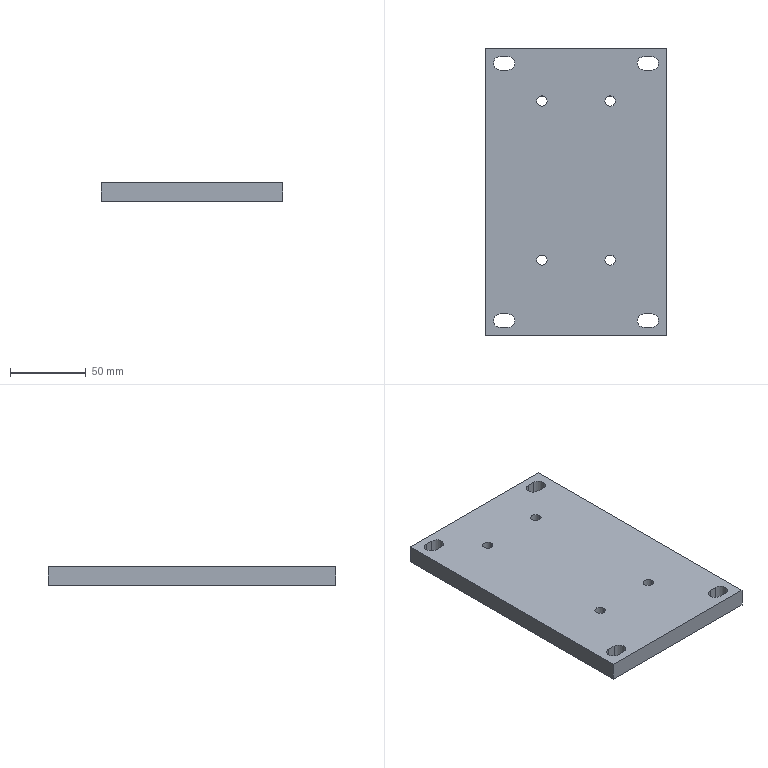Part | STEP file | X77-08202 | 1 solid | 44 faces | box 120 x 190 x 12 mm | volume 260641 mm3 | cylinder 24 | plane 20 | commonest cylinder face diameters 9 x12 6.8 x8 8 x4
STEP:
#1=CARTESIAN_POINT('',(25.9,-643.608,12.));
#2=VERTEX_POINT('',#1);
#3=CARTESIAN_POINT('',(19.1,-643.608,12.));
#4=VERTEX_POINT('',#3);
#5=CARTESIAN_POINT('',(22.5,-643.608,12.));
#6=DIRECTION('',(0.,0.,-1.));
#7=DIRECTION('',(-1.,0.,0.));
#8=AXIS2_PLACEMENT_3D('',#5,#6,#7);
#9=CIRCLE('',#8,3.4);
#10=EDGE_CURVE('',#2,#4,#9,.T.);
#11=ORIENTED_EDGE('',*,*,#10,.F.);
#12=CARTESIAN_POINT('',(25.9,-643.608,2.5));
#13=VERTEX_POINT('',#12);
#14=CARTESIAN_POINT('',(25.9,-643.608,2.5));
#15=DIRECTION('',(0.,0.,-1.));
#16=VECTOR('',#15,1000.);
#17=LINE('',#14,#16);
#18=EDGE_CURVE('',#2,#13,#17,.T.);
#19=ORIENTED_EDGE('',*,*,#18,.T.);
#20=CARTESIAN_POINT('',(19.1,-643.608,2.5));
#21=VERTEX_POINT('',#20);
#22=CARTESIAN_POINT('',(22.5,-643.608,2.5));
#23=DIRECTION('',(0.,0.,-1.));
#24=DIRECTION('',(-1.,0.,0.));
#25=AXIS2_PLACEMENT_3D('',#22,#23,#24);
#26=CIRCLE('',#25,3.4);
#27=EDGE_CURVE('',#13,#21,#26,.T.);
#28=ORIENTED_EDGE('',*,*,#27,.T.);
#29=CARTESIAN_POINT('',(19.1,-643.608,2.5));
#30=DIRECTION('',(0.,0.,-1.));
#31=VECTOR('',#30,1000.);
#32=LINE('',#29,#31);
#33=EDGE_CURVE('',#4,#21,#32,.T.);
#34=ORIENTED_EDGE('',*,*,#33,.F.);
#35=EDGE_LOOP('',(#11,#19,#28,#34));
#36=FACE_OUTER_BOUND('',#35,.T.);
#37=CARTESIAN_POINT('',(22.5,-643.608,2.5));
#38=DIRECTION('',(0.,0.,-1.));
#39=DIRECTION('',(-1.,0.,0.));
#40=AXIS2_PLACEMENT_3D('',#37,#38,#39);
#41=CYLINDRICAL_SURFACE('',#40,3.4);
#42=ADVANCED_FACE('',(#36),#41,.F.);
#43=CARTESIAN_POINT('',(-19.1,-643.601,12.));
#44=VERTEX_POINT('',#43);
#45=CARTESIAN_POINT('',(-25.9,-643.601,12.));
#46=VERTEX_POINT('',#45);
#47=CARTESIAN_POINT('',(-22.5,-643.601,12.));
#48=DIRECTION('',(0.,0.,-1.));
#49=DIRECTION('',(-1.,0.,0.));
#50=AXIS2_PLACEMENT_3D('',#47,#48,#49);
#51=CIRCLE('',#50,3.4);
#52=EDGE_CURVE('',#44,#46,#51,.T.);
#53=ORIENTED_EDGE('',*,*,#52,.F.);
#54=CARTESIAN_POINT('',(-19.1,-643.601,2.5));
#55=VERTEX_POINT('',#54);
#56=CARTESIAN_POINT('',(-19.1,-643.601,2.5));
#57=DIRECTION('',(0.,0.,-1.));
#58=VECTOR('',#57,1000.);
#59=LINE('',#56,#58);
#60=EDGE_CURVE('',#44,#55,#59,.T.);
#61=ORIENTED_EDGE('',*,*,#60,.T.);
#62=CARTESIAN_POINT('',(-25.9,-643.601,2.5));
#63=VERTEX_POINT('',#62);
#64=CARTESIAN_POINT('',(-22.5,-643.601,2.5));
#65=DIRECTION('',(0.,0.,-1.));
#66=DIRECTION('',(-1.,0.,0.));
#67=AXIS2_PLACEMENT_3D('',#64,#65,#66);
#68=CIRCLE('',#67,3.4);
#69=EDGE_CURVE('',#55,#63,#68,.T.);
#70=ORIENTED_EDGE('',*,*,#69,.T.);
#71=CARTESIAN_POINT('',(-25.9,-643.601,2.5));
#72=DIRECTION('',(0.,0.,-1.));
#73=VECTOR('',#72,1000.);
#74=LINE('',#71,#73);
#75=EDGE_CURVE('',#46,#63,#74,.T.);
#76=ORIENTED_EDGE('',*,*,#75,.F.);
#77=EDGE_LOOP('',(#53,#61,#70,#76));
#78=FACE_OUTER_BOUND('',#77,.T.);
#79=CARTESIAN_POINT('',(-22.5,-643.601,2.5));
#80=DIRECTION('',(0.,0.,-1.));
#81=DIRECTION('',(-1.,0.,0.));
#82=AXIS2_PLACEMENT_3D('',#79,#80,#81);
#83=CYLINDRICAL_SURFACE('',#82,3.4);
#84=ADVANCED_FACE('',(#78),#83,.F.);
#85=CARTESIAN_POINT('',(-19.1,-538.608,12.));
#86=VERTEX_POINT('',#85);
#87=CARTESIAN_POINT('',(-25.9,-538.608,12.));
#88=VERTEX_POINT('',#87);
#89=CARTESIAN_POINT('',(-22.5,-538.608,12.));
#90=DIRECTION('',(0.,0.,-1.));
#91=DIRECTION('',(-1.,0.,0.));
#92=AXIS2_PLACEMENT_3D('',#89,#90,#91);
#93=CIRCLE('',#92,3.4);
#94=EDGE_CURVE('',#86,#88,#93,.T.);
#95=ORIENTED_EDGE('',*,*,#94,.F.);
#96=CARTESIAN_POINT('',(-19.1,-538.608,2.5));
#97=VERTEX_POINT('',#96);
#98=CARTESIAN_POINT('',(-19.1,-538.608,2.5));
#99=DIRECTION('',(0.,0.,-1.));
#100=VECTOR('',#99,1000.);
#101=LINE('',#98,#100);
#102=EDGE_CURVE('',#86,#97,#101,.T.);
#103=ORIENTED_EDGE('',*,*,#102,.T.);
#104=CARTESIAN_POINT('',(-25.9,-538.608,2.5));
#105=VERTEX_POINT('',#104);
#106=CARTESIAN_POINT('',(-22.5,-538.608,2.5));
#107=DIRECTION('',(0.,0.,-1.));
#108=DIRECTION('',(-1.,0.,0.));
#109=AXIS2_PLACEMENT_3D('',#106,#107,#108);
#110=CIRCLE('',#109,3.4);
#111=EDGE_CURVE('',#97,#105,#110,.T.);
#112=ORIENTED_EDGE('',*,*,#111,.T.);
#113=CARTESIAN_POINT('',(-25.9,-538.608,2.5));
#114=DIRECTION('',(0.,0.,-1.));
#115=VECTOR('',#114,1000.);
#116=LINE('',#113,#115);
#117=EDGE_CURVE('',#88,#105,#116,.T.);
#118=ORIENTED_EDGE('',*,*,#117,.F.);
#119=EDGE_LOOP('',(#95,#103,#112,#118));
#120=FACE_OUTER_BOUND('',#119,.T.);
#121=CARTESIAN_POINT('',(-22.5,-538.608,2.5));
#122=DIRECTION('',(0.,0.,-1.));
#123=DIRECTION('',(-1.,0.,0.));
#124=AXIS2_PLACEMENT_3D('',#121,#122,#123);
#125=CYLINDRICAL_SURFACE('',#124,3.4);
#126=ADVANCED_FACE('',(#120),#125,.F.);
#127=CARTESIAN_POINT('',(25.9,-538.608,12.));
#128=VERTEX_POINT('',#127);
#129=CARTESIAN_POINT('',(19.1,-538.608,12.));
#130=VERTEX_POINT('',#129);
#131=CARTESIAN_POINT('',(22.5,-538.608,12.));
#132=DIRECTION('',(0.,0.,-1.));
#133=DIRECTION('',(-1.,0.,0.));
#134=AXIS2_PLACEMENT_3D('',#131,#132,#133);
#135=CIRCLE('',#134,3.4);
#136=EDGE_CURVE('',#128,#130,#135,.T.);
#137=ORIENTED_EDGE('',*,*,#136,.F.);
#138=CARTESIAN_POINT('',(25.9,-538.608,2.5));
#139=VERTEX_POINT('',#138);
#140=CARTESIAN_POINT('',(25.9,-538.608,2.5));
#141=DIRECTION('',(0.,0.,-1.));
#142=VECTOR('',#141,1000.);
#143=LINE('',#140,#142);
#144=EDGE_CURVE('',#128,#139,#143,.T.);
#145=ORIENTED_EDGE('',*,*,#144,.T.);
#146=CARTESIAN_POINT('',(19.1,-538.608,2.5));
#147=VERTEX_POINT('',#146);
#148=CARTESIAN_POINT('',(22.5,-538.608,2.5));
#149=DIRECTION('',(0.,0.,-1.));
#150=DIRECTION('',(-1.,0.,0.));
#151=AXIS2_PLACEMENT_3D('',#148,#149,#150);
#152=CIRCLE('',#151,3.4);
#153=EDGE_CURVE('',#139,#147,#152,.T.);
#154=ORIENTED_EDGE('',*,*,#153,.T.);
#155=CARTESIAN_POINT('',(19.1,-538.608,2.5));
#156=DIRECTION('',(0.,0.,-1.));
#157=VECTOR('',#156,1000.);
#158=LINE('',#155,#157);
#159=EDGE_CURVE('',#130,#147,#158,.T.);
#160=ORIENTED_EDGE('',*,*,#159,.F.);
#161=EDGE_LOOP('',(#137,#145,#154,#160));
#162=FACE_OUTER_BOUND('',#161,.T.);
#163=CARTESIAN_POINT('',(22.5,-538.608,2.5));
#164=DIRECTION('',(0.,0.,-1.));
#165=DIRECTION('',(-1.,0.,0.));
#166=AXIS2_PLACEMENT_3D('',#163,#164,#165);
#167=CYLINDRICAL_SURFACE('',#166,3.4);
#168=ADVANCED_FACE('',(#162),#167,.F.);
#169=CARTESIAN_POINT('',(-50.028,-679.108,12.));
#170=VERTEX_POINT('',#169);
#171=CARTESIAN_POINT('',(-54.528,-683.608,12.));
#172=VERTEX_POINT('',#171);
#173=CARTESIAN_POINT('',(-50.028,-683.608,12.));
#174=DIRECTION('',(0.,0.,1.));
#175=DIRECTION('',(-1.,0.,0.));
#176=AXIS2_PLACEMENT_3D('',#173,#174,#175);
#177=CIRCLE('',#176,4.5);
#178=EDGE_CURVE('',#170,#172,#177,.T.);
#179=ORIENTED_EDGE('',*,*,#178,.T.);
#180=CARTESIAN_POINT('',(-54.528,-683.608,0.));
#181=VERTEX_POINT('',#180);
#182=CARTESIAN_POINT('',(-54.528,-683.608,12.));
#183=DIRECTION('',(0.,0.,-1.));
#184=VECTOR('',#183,1000.);
#185=LINE('',#182,#184);
#186=EDGE_CURVE('',#172,#181,#185,.T.);
#187=ORIENTED_EDGE('',*,*,#186,.T.);
#188=CARTESIAN_POINT('',(-50.028,-679.108,0.));
#189=VERTEX_POINT('',#188);
#190=CARTESIAN_POINT('',(-50.028,-683.608,0.));
#191=DIRECTION('',(0.,0.,1.));
#192=DIRECTION('',(-1.,0.,0.));
#193=AXIS2_PLACEMENT_3D('',#190,#191,#192);
#194=CIRCLE('',#193,4.5);
#195=EDGE_CURVE('',#189,#181,#194,.T.);
#196=ORIENTED_EDGE('',*,*,#195,.F.);
#197=CARTESIAN_POINT('',(-50.028,-679.108,12.));
#198=DIRECTION('',(0.,0.,-1.));
#199=VECTOR('',#198,1000.);
#200=LINE('',#197,#199);
#201=EDGE_CURVE('',#170,#189,#200,.T.);
#202=ORIENTED_EDGE('',*,*,#201,.F.);
#203=EDGE_LOOP('',(#179,#187,#196,#202));
#204=FACE_OUTER_BOUND('',#203,.T.);
#205=CARTESIAN_POINT('',(-50.028,-683.608,12.));
#206=DIRECTION('',(0.,0.,-1.));
#207=DIRECTION('',(-1.,0.,0.));
#208=AXIS2_PLACEMENT_3D('',#205,#206,#207);
#209=CYLINDRICAL_SURFACE('',#208,4.5);
#210=ADVANCED_FACE('',(#204),#209,.F.);
#211=CARTESIAN_POINT('',(44.972,-679.108,12.));
#212=VERTEX_POINT('',#211);
#213=CARTESIAN_POINT('',(40.472,-683.608,12.));
#214=VERTEX_POINT('',#213);
#215=CARTESIAN_POINT('',(44.972,-683.608,12.));
#216=DIRECTION('',(0.,0.,1.));
#217=DIRECTION('',(1.,0.,0.));
#218=AXIS2_PLACEMENT_3D('',#215,#216,#217);
#219=CIRCLE('',#218,4.5);
#220=EDGE_CURVE('',#212,#214,#219,.T.);
#221=ORIENTED_EDGE('',*,*,#220,.T.);
#222=CARTESIAN_POINT('',(40.472,-683.608,0.));
#223=VERTEX_POINT('',#222);
#224=CARTESIAN_POINT('',(40.472,-683.608,12.));
#225=DIRECTION('',(0.,0.,-1.));
#226=VECTOR('',#225,1000.);
#227=LINE('',#224,#226);
#228=EDGE_CURVE('',#214,#223,#227,.T.);
#229=ORIENTED_EDGE('',*,*,#228,.T.);
#230=CARTESIAN_POINT('',(44.972,-679.108,0.));
#231=VERTEX_POINT('',#230);
#232=CARTESIAN_POINT('',(44.972,-683.608,0.));
#233=DIRECTION('',(0.,0.,1.));
#234=DIRECTION('',(1.,0.,0.));
#235=AXIS2_PLACEMENT_3D('',#232,#233,#234);
#236=CIRCLE('',#235,4.5);
#237=EDGE_CURVE('',#231,#223,#236,.T.);
#238=ORIENTED_EDGE('',*,*,#237,.F.);
#239=CARTESIAN_POINT('',(44.972,-679.108,12.));
#240=DIRECTION('',(0.,0.,-1.));
#241=VECTOR('',#240,1000.);
#242=LINE('',#239,#241);
#243=EDGE_CURVE('',#212,#231,#242,.T.);
#244=ORIENTED_EDGE('',*,*,#243,.F.);
#245=EDGE_LOOP('',(#221,#229,#238,#244));
#246=FACE_OUTER_BOUND('',#245,.T.);
#247=CARTESIAN_POINT('',(44.972,-683.608,12.));
#248=DIRECTION('',(0.,0.,-1.));
#249=DIRECTION('',(-1.,0.,0.));
#250=AXIS2_PLACEMENT_3D('',#247,#248,#249);
#251=CYLINDRICAL_SURFACE('',#250,4.5);
#252=ADVANCED_FACE('',(#246),#251,.F.);
#253=CARTESIAN_POINT('',(44.972,-509.108,12.));
#254=VERTEX_POINT('',#253);
#255=CARTESIAN_POINT('',(40.472,-513.608,12.));
#256=VERTEX_POINT('',#255);
#257=CARTESIAN_POINT('',(44.972,-513.608,12.));
#258=DIRECTION('',(0.,0.,1.));
#259=DIRECTION('',(-1.,0.,0.));
#260=AXIS2_PLACEMENT_3D('',#257,#258,#259);
#261=CIRCLE('',#260,4.5);
#262=EDGE_CURVE('',#254,#256,#261,.T.);
#263=ORIENTED_EDGE('',*,*,#262,.T.);
#264=CARTESIAN_POINT('',(40.472,-513.608,0.));
#265=VERTEX_POINT('',#264);
#266=CARTESIAN_POINT('',(40.472,-513.608,12.));
#267=DIRECTION('',(0.,0.,-1.));
#268=VECTOR('',#267,1000.);
#269=LINE('',#266,#268);
#270=EDGE_CURVE('',#256,#265,#269,.T.);
#271=ORIENTED_EDGE('',*,*,#270,.T.);
#272=CARTESIAN_POINT('',(44.972,-509.108,0.));
#273=VERTEX_POINT('',#272);
#274=CARTESIAN_POINT('',(44.972,-513.608,0.));
#275=DIRECTION('',(0.,0.,1.));
#276=DIRECTION('',(-1.,0.,0.));
#277=AXIS2_PLACEMENT_3D('',#274,#275,#276);
#278=CIRCLE('',#277,4.5);
#279=EDGE_CURVE('',#273,#265,#278,.T.);
#280=ORIENTED_EDGE('',*,*,#279,.F.);
#281=CARTESIAN_POINT('',(44.972,-509.108,12.));
#282=DIRECTION('',(0.,0.,-1.));
#283=VECTOR('',#282,1000.);
#284=LINE('',#281,#283);
#285=EDGE_CURVE('',#254,#273,#284,.T.);
#286=ORIENTED_EDGE('',*,*,#285,.F.);
#287=EDGE_LOOP('',(#263,#271,#280,#286));
#288=FACE_OUTER_BOUND('',#287,.T.);
#289=CARTESIAN_POINT('',(44.972,-513.608,12.));
#290=DIRECTION('',(0.,0.,-1.));
#291=DIRECTION('',(-1.,0.,0.));
#292=AXIS2_PLACEMENT_3D('',#289,#290,#291);
#293=CYLINDRICAL_SURFACE('',#292,4.5);
#294=ADVANCED_FACE('',(#288),#293,.F.);
#295=CARTESIAN_POINT('',(-50.028,-509.108,12.));
#296=VERTEX_POINT('',#295);
#297=CARTESIAN_POINT('',(-54.528,-513.608,12.));
#298=VERTEX_POINT('',#297);
#299=CARTESIAN_POINT('',(-50.028,-513.608,12.));
#300=DIRECTION('',(0.,0.,1.));
#301=DIRECTION('',(1.,0.,0.));
#302=AXIS2_PLACEMENT_3D('',#299,#300,#301);
#303=CIRCLE('',#302,4.5);
#304=EDGE_CURVE('',#296,#298,#303,.T.);
#305=ORIENTED_EDGE('',*,*,#304,.T.);
#306=CARTESIAN_POINT('',(-54.528,-513.608,0.));
#307=VERTEX_POINT('',#306);
#308=CARTESIAN_POINT('',(-54.528,-513.608,12.));
#309=DIRECTION('',(0.,0.,-1.));
#310=VECTOR('',#309,1000.);
#311=LINE('',#308,#310);
#312=EDGE_CURVE('',#298,#307,#311,.T.);
#313=ORIENTED_EDGE('',*,*,#312,.T.);
#314=CARTESIAN_POINT('',(-50.028,-509.108,0.));
#315=VERTEX_POINT('',#314);
#316=CARTESIAN_POINT('',(-50.028,-513.608,0.));
#317=DIRECTION('',(0.,0.,1.));
#318=DIRECTION('',(1.,0.,0.));
#319=AXIS2_PLACEMENT_3D('',#316,#317,#318);
#320=CIRCLE('',#319,4.5);
#321=EDGE_CURVE('',#315,#307,#320,.T.);
#322=ORIENTED_EDGE('',*,*,#321,.F.);
#323=CARTESIAN_POINT('',(-50.028,-509.108,12.));
#324=DIRECTION('',(0.,0.,-1.));
#325=VECTOR('',#324,1000.);
#326=LINE('',#323,#325);
#327=EDGE_CURVE('',#296,#315,#326,.T.);
#328=ORIENTED_EDGE('',*,*,#327,.F.);
#329=EDGE_LOOP('',(#305,#313,#322,#328));
#330=FACE_OUTER_BOUND('',#329,.T.);
#331=CARTESIAN_POINT('',(-50.028,-513.608,12.));
#332=DIRECTION('',(0.,0.,-1.));
#333=DIRECTION('',(-1.,0.,0.));
#334=AXIS2_PLACEMENT_3D('',#331,#332,#333);
#335=CYLINDRICAL_SURFACE('',#334,4.5);
#336=ADVANCED_FACE('',(#330),#335,.F.);
#337=CARTESIAN_POINT('',(22.5,-643.608,12.));
#338=DIRECTION('',(0.,0.,-1.));
#339=DIRECTION('',(-1.,0.,0.));
#340=AXIS2_PLACEMENT_3D('',#337,#338,#339);
#341=CIRCLE('',#340,3.4);
#342=EDGE_CURVE('',#4,#2,#341,.T.);
#343=ORIENTED_EDGE('',*,*,#342,.T.);
#344=ORIENTED_EDGE('',*,*,#10,.T.);
#345=EDGE_LOOP('',(#343,#344));
#346=FACE_BOUND('',#345,.T.);
#347=CARTESIAN_POINT('',(-22.5,-643.601,12.));
#348=DIRECTION('',(0.,0.,-1.));
#349=DIRECTION('',(-1.,0.,0.));
#350=AXIS2_PLACEMENT_3D('',#347,#348,#349);
#351=CIRCLE('',#350,3.4);
#352=EDGE_CURVE('',#46,#44,#351,.T.);
#353=ORIENTED_EDGE('',*,*,#352,.T.);
#354=ORIENTED_EDGE('',*,*,#52,.T.);
#355=EDGE_LOOP('',(#353,#354));
#356=FACE_BOUND('',#355,.T.);
#357=CARTESIAN_POINT('',(-22.5,-538.608,12.));
#358=DIRECTION('',(0.,0.,-1.));
#359=DIRECTION('',(-1.,0.,0.));
#360=AXIS2_PLACEMENT_3D('',#357,#358,#359);
#361=CIRCLE('',#360,3.4);
#362=EDGE_CURVE('',#88,#86,#361,.T.);
#363=ORIENTED_EDGE('',*,*,#362,.T.);
#364=ORIENTED_EDGE('',*,*,#94,.T.);
#365=EDGE_LOOP('',(#363,#364));
#366=FACE_BOUND('',#365,.T.);
#367=CARTESIAN_POINT('',(22.5,-538.608,12.));
#368=DIRECTION('',(0.,0.,-1.));
#369=DIRECTION('',(-1.,0.,0.));
#370=AXIS2_PLACEMENT_3D('',#367,#368,#369);
#371=CIRCLE('',#370,3.4);
#372=EDGE_CURVE('',#130,#128,#371,.T.);
#373=ORIENTED_EDGE('',*,*,#372,.T.);
#374=ORIENTED_EDGE('',*,*,#136,.T.);
#375=EDGE_LOOP('',(#373,#374));
#376=FACE_BOUND('',#375,.T.);
#377=CARTESIAN_POINT('',(49.972,-688.108,12.));
#378=VERTEX_POINT('',#377);
#379=CARTESIAN_POINT('',(49.972,-679.108,12.));
#380=VERTEX_POINT('',#379);
#381=CARTESIAN_POINT('',(49.972,-683.608,12.));
#382=DIRECTION('',(0.,0.,1.));
#383=DIRECTION('',(1.,0.,0.));
#384=AXIS2_PLACEMENT_3D('',#381,#382,#383);
#385=CIRCLE('',#384,4.5);
#386=EDGE_CURVE('',#378,#380,#385,.T.);
#387=ORIENTED_EDGE('',*,*,#386,.F.);
#388=CARTESIAN_POINT('',(44.972,-688.108,12.));
#389=VERTEX_POINT('',#388);
#390=CARTESIAN_POINT('',(49.972,-688.108,12.));
#391=DIRECTION('',(1.,0.,0.));
#392=VECTOR('',#391,1000.);
#393=LINE('',#390,#392);
#394=EDGE_CURVE('',#389,#378,#393,.T.);
#395=ORIENTED_EDGE('',*,*,#394,.F.);
#396=CARTESIAN_POINT('',(44.972,-683.608,12.));
#397=DIRECTION('',(0.,0.,1.));
#398=DIRECTION('',(1.,0.,0.));
#399=AXIS2_PLACEMENT_3D('',#396,#397,#398);
#400=CIRCLE('',#399,4.5);
#401=EDGE_CURVE('',#214,#389,#400,.T.);
#402=ORIENTED_EDGE('',*,*,#401,.F.);
#403=ORIENTED_EDGE('',*,*,#220,.F.);
#404=CARTESIAN_POINT('',(49.972,-679.108,12.));
#405=DIRECTION('',(-1.,0.,0.));
#406=VECTOR('',#405,1000.);
#407=LINE('',#404,#406);
#408=EDGE_CURVE('',#380,#212,#407,.T.);
#409=ORIENTED_EDGE('',*,*,#408,.F.);
#410=EDGE_LOOP('',(#387,#395,#402,#403,#409));
#411=FACE_BOUND('',#410,.T.);
#412=ORIENTED_EDGE('',*,*,#304,.F.);
#413=CARTESIAN_POINT('',(-45.028,-509.108,12.));
#414=VERTEX_POINT('',#413);
#415=CARTESIAN_POINT('',(-50.028,-509.108,12.));
#416=DIRECTION('',(-1.,0.,0.));
#417=VECTOR('',#416,1000.);
#418=LINE('',#415,#417);
#419=EDGE_CURVE('',#414,#296,#418,.T.);
#420=ORIENTED_EDGE('',*,*,#419,.F.);
#421=CARTESIAN_POINT('',(-45.028,-518.108,12.));
#422=VERTEX_POINT('',#421);
#423=CARTESIAN_POINT('',(-45.028,-513.608,12.));
#424=DIRECTION('',(0.,0.,1.));
#425=DIRECTION('',(1.,0.,0.));
#426=AXIS2_PLACEMENT_3D('',#423,#424,#425);
#427=CIRCLE('',#426,4.5);
#428=EDGE_CURVE('',#422,#414,#427,.T.);
#429=ORIENTED_EDGE('',*,*,#428,.F.);
#430=CARTESIAN_POINT('',(-50.028,-518.108,12.));
#431=VERTEX_POINT('',#430);
#432=CARTESIAN_POINT('',(-50.028,-518.108,12.));
#433=DIRECTION('',(1.,0.,0.));
#434=VECTOR('',#433,1000.);
#435=LINE('',#432,#434);
#436=EDGE_CURVE('',#431,#422,#435,.T.);
#437=ORIENTED_EDGE('',*,*,#436,.F.);
#438=CARTESIAN_POINT('',(-50.028,-513.608,12.));
#439=DIRECTION('',(0.,0.,1.));
#440=DIRECTION('',(1.,0.,0.));
#441=AXIS2_PLACEMENT_3D('',#438,#439,#440);
#442=CIRCLE('',#441,4.5);
#443=EDGE_CURVE('',#298,#431,#442,.T.);
#444=ORIENTED_EDGE('',*,*,#443,.F.);
#445=EDGE_LOOP('',(#412,#420,#429,#437,#444));
#446=FACE_BOUND('',#445,.T.);
#447=CARTESIAN_POINT('',(-60.028,-503.608,12.));
#448=VERTEX_POINT('',#447);
#449=CARTESIAN_POINT('',(-60.028,-693.608,12.));
#450=VERTEX_POINT('',#449);
#451=CARTESIAN_POINT('',(-60.028,-693.608,12.));
#452=DIRECTION('',(0.,-1.,0.));
#453=VECTOR('',#452,1000.);
#454=LINE('',#451,#453);
#455=EDGE_CURVE('',#448,#450,#454,.T.);
#456=ORIENTED_EDGE('',*,*,#455,.T.);
#457=CARTESIAN_POINT('',(59.972,-693.608,12.));
#458=VERTEX_POINT('',#457);
#459=CARTESIAN_POINT('',(-60.028,-693.608,12.));
#460=DIRECTION('',(1.,0.,0.));
#461=VECTOR('',#460,1000.);
#462=LINE('',#459,#461);
#463=EDGE_CURVE('',#450,#458,#462,.T.);
#464=ORIENTED_EDGE('',*,*,#463,.T.);
#465=CARTESIAN_POINT('',(59.972,-503.608,12.));
#466=VERTEX_POINT('',#465);
#467=CARTESIAN_POINT('',(59.972,-693.608,12.));
#468=DIRECTION('',(0.,1.,0.));
#469=VECTOR('',#468,1000.);
#470=LINE('',#467,#469);
#471=EDGE_CURVE('',#458,#466,#470,.T.);
#472=ORIENTED_EDGE('',*,*,#471,.T.);
#473=CARTESIAN_POINT('',(-60.028,-503.608,12.));
#474=DIRECTION('',(-1.,0.,0.));
#475=VECTOR('',#474,1000.);
#476=LINE('',#473,#475);
#477=EDGE_CURVE('',#466,#448,#476,.T.);
#478=ORIENTED_EDGE('',*,*,#477,.T.);
#479=EDGE_LOOP('',(#456,#464,#472,#478));
#480=FACE_OUTER_BOUND('',#479,.T.);
#481=CARTESIAN_POINT('',(49.972,-518.108,12.));
#482=VERTEX_POINT('',#481);
#483=CARTESIAN_POINT('',(49.972,-509.108,12.));
#484=VERTEX_POINT('',#483);
#485=CARTESIAN_POINT('',(49.972,-513.608,12.));
#486=DIRECTION('',(0.,0.,1.));
#487=DIRECTION('',(-1.,0.,0.));
#488=AXIS2_PLACEMENT_3D('',#485,#486,#487);
#489=CIRCLE('',#488,4.5);
#490=EDGE_CURVE('',#482,#484,#489,.T.);
#491=ORIENTED_EDGE('',*,*,#490,.F.);
#492=CARTESIAN_POINT('',(44.972,-518.108,12.));
#493=VERTEX_POINT('',#492);
#494=CARTESIAN_POINT('',(49.972,-518.108,12.));
#495=DIRECTION('',(1.,0.,0.));
#496=VECTOR('',#495,1000.);
#497=LINE('',#494,#496);
#498=EDGE_CURVE('',#493,#482,#497,.T.);
#499=ORIENTED_EDGE('',*,*,#498,.F.);
#500=CARTESIAN_POINT('',(44.972,-513.608,12.));
#501=DIRECTION('',(0.,0.,1.));
#502=DIRECTION('',(-1.,0.,0.));
#503=AXIS2_PLACEMENT_3D('',#500,#501,#502);
#504=CIRCLE('',#503,4.5);
#505=EDGE_CURVE('',#256,#493,#504,.T.);
#506=ORIENTED_EDGE('',*,*,#505,.F.);
#507=ORIENTED_EDGE('',*,*,#262,.F.);
#508=CARTESIAN_POINT('',(49.972,-509.108,12.));
#509=DIRECTION('',(-1.,0.,0.));
#510=VECTOR('',#509,1000.);
#511=LINE('',#508,#510);
#512=EDGE_CURVE('',#484,#254,#511,.T.);
#513=ORIENTED_EDGE('',*,*,#512,.F.);
#514=EDGE_LOOP('',(#491,#499,#506,#507,#513));
#515=FACE_BOUND('',#514,.T.);
#516=ORIENTED_EDGE('',*,*,#178,.F.);
#517=CARTESIAN_POINT('',(-45.028,-679.108,12.));
#518=VERTEX_POINT('',#517);
#519=CARTESIAN_POINT('',(-50.028,-679.108,12.));
#520=DIRECTION('',(-1.,0.,0.));
#521=VECTOR('',#520,1000.);
#522=LINE('',#519,#521);
#523=EDGE_CURVE('',#518,#170,#522,.T.);
#524=ORIENTED_EDGE('',*,*,#523,.F.);
#525=CARTESIAN_POINT('',(-45.028,-688.108,12.));
#526=VERTEX_POINT('',#525);
#527=CARTESIAN_POINT('',(-45.028,-683.608,12.));
#528=DIRECTION('',(0.,0.,1.));
#529=DIRECTION('',(-1.,0.,0.));
#530=AXIS2_PLACEMENT_3D('',#527,#528,#529);
#531=CIRCLE('',#530,4.5);
#532=EDGE_CURVE('',#526,#518,#531,.T.);
#533=ORIENTED_EDGE('',*,*,#532,.F.);
#534=CARTESIAN_POINT('',(-50.028,-688.108,12.));
#535=VERTEX_POINT('',#534);
#536=CARTESIAN_POINT('',(-50.028,-688.108,12.));
#537=DIRECTION('',(1.,0.,0.));
#538=VECTOR('',#537,1000.);
#539=LINE('',#536,#538);
#540=EDGE_CURVE('',#535,#526,#539,.T.);
#541=ORIENTED_EDGE('',*,*,#540,.F.);
#542=CARTESIAN_POINT('',(-50.028,-683.608,12.));
#543=DIRECTION('',(0.,0.,1.));
#544=DIRECTION('',(-1.,0.,0.));
#545=AXIS2_PLACEMENT_3D('',#542,#543,#544);
#546=CIRCLE('',#545,4.5);
#547=EDGE_CURVE('',#172,#535,#546,.T.);
#548=ORIENTED_EDGE('',*,*,#547,.F.);
#549=EDGE_LOOP('',(#516,#524,#533,#541,#548));
#550=FACE_BOUND('',#549,.T.);
#551=CARTESIAN_POINT('',(-60.028,-503.608,12.));
#552=DIRECTION('',(0.,0.,-1.));
#553=DIRECTION('',(-1.,0.,0.));
#554=AXIS2_PLACEMENT_3D('',#551,#552,#553);
#555=PLANE('',#554);
#556=ADVANCED_FACE('',(#346,#356,#366,#376,#411,#446,#480,#515,#550),#555,.F.);
#557=CARTESIAN_POINT('',(18.497,-659.608,0.));
#558=VERTEX_POINT('',#557);
#559=CARTESIAN_POINT('',(22.497,-663.608,0.));
#560=VERTEX_POINT('',#559);
#561=CARTESIAN_POINT('',(22.497,-659.608,0.));
#562=DIRECTION('',(0.,0.,1.));
#563=DIRECTION('',(-1.,0.,0.));
#564=AXIS2_PLACEMENT_3D('',#561,#562,#563);
#565=CIRCLE('',#564,4.);
#566=EDGE_CURVE('',#558,#560,#565,.T.);
#567=ORIENTED_EDGE('',*,*,#566,.T.);
#568=CARTESIAN_POINT('',(26.497,-659.608,0.));
#569=VERTEX_POINT('',#568);
#570=CARTESIAN_POINT('',(22.497,-659.608,0.));
#571=DIRECTION('',(0.,0.,1.));
#572=DIRECTION('',(-1.,0.,0.));
#573=AXIS2_PLACEMENT_3D('',#570,#571,#572);
#574=CIRCLE('',#573,4.);
#575=EDGE_CURVE('',#560,#569,#574,.T.);
#576=ORIENTED_EDGE('',*,*,#575,.T.);
#577=CARTESIAN_POINT('',(26.497,-503.608,0.));
#578=VERTEX_POINT('',#577);
#579=CARTESIAN_POINT('',(26.497,-663.608,0.));
#580=DIRECTION('',(0.,1.,0.));
#581=VECTOR('',#580,1000.);
#582=LINE('',#579,#581);
#583=EDGE_CURVE('',#569,#578,#582,.T.);
#584=ORIENTED_EDGE('',*,*,#583,.T.);
#585=CARTESIAN_POINT('',(59.972,-503.608,0.));
#586=VERTEX_POINT('',#585);
#587=CARTESIAN_POINT('',(-60.028,-503.608,0.));
#588=DIRECTION('',(-1.,0.,0.));
#589=VECTOR('',#588,1000.);
#590=LINE('',#587,#589);
#591=EDGE_CURVE('',#586,#578,#590,.T.);
#592=ORIENTED_EDGE('',*,*,#591,.F.);
#593=CARTESIAN_POINT('',(59.972,-693.608,0.));
#594=VERTEX_POINT('',#593);
#595=CARTESIAN_POINT('',(59.972,-693.608,0.));
#596=DIRECTION('',(0.,1.,0.));
#597=VECTOR('',#596,1000.);
#598=LINE('',#595,#597);
#599=EDGE_CURVE('',#594,#586,#598,.T.);
#600=ORIENTED_EDGE('',*,*,#599,.F.);
#601=CARTESIAN_POINT('',(-60.028,-693.608,0.));
#602=VERTEX_POINT('',#601);
#603=CARTESIAN_POINT('',(-60.028,-693.608,0.));
#604=DIRECTION('',(1.,0.,0.));
#605=VECTOR('',#604,1000.);
#606=LINE('',#603,#605);
#607=EDGE_CURVE('',#602,#594,#606,.T.);
#608=ORIENTED_EDGE('',*,*,#607,.F.);
#609=CARTESIAN_POINT('',(-60.028,-503.608,0.));
#610=VERTEX_POINT('',#609);
#611=CARTESIAN_POINT('',(-60.028,-693.608,0.));
#612=DIRECTION('',(0.,-1.,0.));
#613=VECTOR('',#612,1000.);
#614=LINE('',#611,#613);
#615=EDGE_CURVE('',#610,#602,#614,.T.);
#616=ORIENTED_EDGE('',*,*,#615,.F.);
#617=CARTESIAN_POINT('',(-26.503,-503.608,0.));
#618=VERTEX_POINT('',#617);
#619=CARTESIAN_POINT('',(-60.028,-503.608,0.));
#620=DIRECTION('',(-1.,0.,0.));
#621=VECTOR('',#620,1000.);
#622=LINE('',#619,#621);
#623=EDGE_CURVE('',#618,#610,#622,.T.);
#624=ORIENTED_EDGE('',*,*,#623,.F.);
#625=CARTESIAN_POINT('',(-26.503,-659.608,0.));
#626=VERTEX_POINT('',#625);
#627=CARTESIAN_POINT('',(-26.503,-663.608,0.));
#628=DIRECTION('',(0.,1.,0.));
#629=VECTOR('',#628,1000.);
#630=LINE('',#627,#629);
#631=EDGE_CURVE('',#626,#618,#630,.T.);
#632=ORIENTED_EDGE('',*,*,#631,.F.);
#633=CARTESIAN_POINT('',(-22.503,-663.608,0.));
#634=VERTEX_POINT('',#633);
#635=CARTESIAN_POINT('',(-22.503,-659.608,0.));
#636=DIRECTION('',(0.,0.,1.));
#637=DIRECTION('',(-1.,0.,0.));
#638=AXIS2_PLACEMENT_3D('',#635,#636,#637);
#639=CIRCLE('',#638,4.);
#640=EDGE_CURVE('',#626,#634,#639,.T.);
#641=ORIENTED_EDGE('',*,*,#640,.T.);
#642=CARTESIAN_POINT('',(-18.503,-659.608,0.));
#643=VERTEX_POINT('',#642);
#644=CARTESIAN_POINT('',(-22.503,-659.608,0.));
#645=DIRECTION('',(0.,0.,1.));
#646=DIRECTION('',(-1.,0.,0.));
#647=AXIS2_PLACEMENT_3D('',#644,#645,#646);
#648=CIRCLE('',#647,4.);
#649=EDGE_CURVE('',#634,#643,#648,.T.);
#650=ORIENTED_EDGE('',*,*,#649,.T.);
#651=CARTESIAN_POINT('',(-18.503,-503.608,0.));
#652=VERTEX_POINT('',#651);
#653=CARTESIAN_POINT('',(-18.503,-663.608,0.));
#654=DIRECTION('',(0.,1.,0.));
#655=VECTOR('',#654,1000.);
#656=LINE('',#653,#655);
#657=EDGE_CURVE('',#643,#652,#656,.T.);
#658=ORIENTED_EDGE('',*,*,#657,.T.);
#659=CARTESIAN_POINT('',(18.497,-503.608,0.));
#660=VERTEX_POINT('',#659);
#661=CARTESIAN_POINT('',(-60.028,-503.608,0.));
#662=DIRECTION('',(-1.,0.,0.));
#663=VECTOR('',#662,1000.);
#664=LINE('',#661,#663);
#665=EDGE_CURVE('',#660,#652,#664,.T.);
#666=ORIENTED_EDGE('',*,*,#665,.F.);
#667=CARTESIAN_POINT('',(18.497,-663.608,0.));
#668=DIRECTION('',(0.,1.,0.));
#669=VECTOR('',#668,1000.);
#670=LINE('',#667,#669);
#671=EDGE_CURVE('',#558,#660,#670,.T.);
#672=ORIENTED_EDGE('',*,*,#671,.F.);
#673=EDGE_LOOP('',(#567,#576,#584,#592,#600,#608,#616,#624,#632,#641,#650,#658,#666,#672));
#674=FACE_OUTER_BOUND('',#673,.T.);
#675=CARTESIAN_POINT('',(44.972,-688.108,0.));
#676=VERTEX_POINT('',#675);
#677=CARTESIAN_POINT('',(49.972,-688.108,0.));
#678=VERTEX_POINT('',#677);
#679=CARTESIAN_POINT('',(49.972,-688.108,0.));
#680=DIRECTION('',(1.,0.,0.));
#681=VECTOR('',#680,1000.);
#682=LINE('',#679,#681);
#683=EDGE_CURVE('',#676,#678,#682,.T.);
#684=ORIENTED_EDGE('',*,*,#683,.T.);
#685=CARTESIAN_POINT('',(49.972,-679.108,0.));
#686=VERTEX_POINT('',#685);
#687=CARTESIAN_POINT('',(49.972,-683.608,0.));
#688=DIRECTION('',(0.,0.,1.));
#689=DIRECTION('',(1.,0.,0.));
#690=AXIS2_PLACEMENT_3D('',#687,#688,#689);
#691=CIRCLE('',#690,4.5);
#692=EDGE_CURVE('',#678,#686,#691,.T.);
#693=ORIENTED_EDGE('',*,*,#692,.T.);
#694=CARTESIAN_POINT('',(49.972,-679.108,0.));
#695=DIRECTION('',(-1.,0.,0.));
#696=VECTOR('',#695,1000.);
#697=LINE('',#694,#696);
#698=EDGE_CURVE('',#686,#231,#697,.T.);
#699=ORIENTED_EDGE('',*,*,#698,.T.);
#700=ORIENTED_EDGE('',*,*,#237,.T.);
#701=CARTESIAN_POINT('',(44.972,-683.608,0.));
#702=DIRECTION('',(0.,0.,1.));
#703=DIRECTION('',(1.,0.,0.));
#704=AXIS2_PLACEMENT_3D('',#701,#702,#703);
#705=CIRCLE('',#704,4.5);
#706=EDGE_CURVE('',#223,#676,#705,.T.);
#707=ORIENTED_EDGE('',*,*,#706,.T.);
#708=EDGE_LOOP('',(#684,#693,#699,#700,#707));
#709=FACE_BOUND('',#708,.T.);
#710=CARTESIAN_POINT('',(-45.028,-509.108,0.));
#711=VERTEX_POINT('',#710);
#712=CARTESIAN_POINT('',(-50.028,-509.108,0.));
#713=DIRECTION('',(-1.,0.,0.));
#714=VECTOR('',#713,1000.);
#715=LINE('',#712,#714);
#716=EDGE_CURVE('',#711,#315,#715,.T.);
#717=ORIENTED_EDGE('',*,*,#716,.T.);
#718=ORIENTED_EDGE('',*,*,#321,.T.);
#719=CARTESIAN_POINT('',(-50.028,-518.108,0.));
#720=VERTEX_POINT('',#719);
#721=CARTESIAN_POINT('',(-50.028,-513.608,0.));
#722=DIRECTION('',(0.,0.,1.));
#723=DIRECTION('',(1.,0.,0.));
#724=AXIS2_PLACEMENT_3D('',#721,#722,#723);
#725=CIRCLE('',#724,4.5);
#726=EDGE_CURVE('',#307,#720,#725,.T.);
#727=ORIENTED_EDGE('',*,*,#726,.T.);
#728=CARTESIAN_POINT('',(-45.028,-518.108,0.));
#729=VERTEX_POINT('',#728);
#730=CARTESIAN_POINT('',(-50.028,-518.108,0.));
#731=DIRECTION('',(1.,0.,0.));
#732=VECTOR('',#731,1000.);
#733=LINE('',#730,#732);
#734=EDGE_CURVE('',#720,#729,#733,.T.);
#735=ORIENTED_EDGE('',*,*,#734,.T.);
#736=CARTESIAN_POINT('',(-45.028,-513.608,0.));
#737=DIRECTION('',(0.,0.,1.));
#738=DIRECTION('',(1.,0.,0.));
#739=AXIS2_PLACEMENT_3D('',#736,#737,#738);
#740=CIRCLE('',#739,4.5);
#741=EDGE_CURVE('',#729,#711,#740,.T.);
#742=ORIENTED_EDGE('',*,*,#741,.T.);
#743=EDGE_LOOP('',(#717,#718,#727,#735,#742));
#744=FACE_BOUND('',#743,.T.);
#745=CARTESIAN_POINT('',(44.972,-518.108,0.));
#746=VERTEX_POINT('',#745);
#747=CARTESIAN_POINT('',(49.972,-518.108,0.));
#748=VERTEX_POINT('',#747);
#749=CARTESIAN_POINT('',(49.972,-518.108,0.));
#750=DIRECTION('',(1.,0.,0.));
#751=VECTOR('',#750,1000.);
#752=LINE('',#749,#751);
#753=EDGE_CURVE('',#746,#748,#752,.T.);
#754=ORIENTED_EDGE('',*,*,#753,.T.);
#755=CARTESIAN_POINT('',(49.972,-509.108,0.));
#756=VERTEX_POINT('',#755);
#757=CARTESIAN_POINT('',(49.972,-513.608,0.));
#758=DIRECTION('',(0.,0.,1.));
#759=DIRECTION('',(-1.,0.,0.));
#760=AXIS2_PLACEMENT_3D('',#757,#758,#759);
#761=CIRCLE('',#760,4.5);
#762=EDGE_CURVE('',#748,#756,#761,.T.);
#763=ORIENTED_EDGE('',*,*,#762,.T.);
#764=CARTESIAN_POINT('',(49.972,-509.108,0.));
#765=DIRECTION('',(-1.,0.,0.));
#766=VECTOR('',#765,1000.);
#767=LINE('',#764,#766);
#768=EDGE_CURVE('',#756,#273,#767,.T.);
#769=ORIENTED_EDGE('',*,*,#768,.T.);
#770=ORIENTED_EDGE('',*,*,#279,.T.);
#771=CARTESIAN_POINT('',(44.972,-513.608,0.));
#772=DIRECTION('',(0.,0.,1.));
#773=DIRECTION('',(-1.,0.,0.));
#774=AXIS2_PLACEMENT_3D('',#771,#772,#773);
#775=CIRCLE('',#774,4.5);
#776=EDGE_CURVE('',#265,#746,#775,.T.);
#777=ORIENTED_EDGE('',*,*,#776,.T.);
#778=EDGE_LOOP('',(#754,#763,#769,#770,#777));
#779=FACE_BOUND('',#778,.T.);
#780=CARTESIAN_POINT('',(-45.028,-679.108,0.));
#781=VERTEX_POINT('',#780);
#782=CARTESIAN_POINT('',(-50.028,-679.108,0.));
#783=DIRECTION('',(-1.,0.,0.));
#784=VECTOR('',#783,1000.);
#785=LINE('',#782,#784);
#786=EDGE_CURVE('',#781,#189,#785,.T.);
#787=ORIENTED_EDGE('',*,*,#786,.T.);
#788=ORIENTED_EDGE('',*,*,#195,.T.);
#789=CARTESIAN_POINT('',(-50.028,-688.108,0.));
#790=VERTEX_POINT('',#789);
#791=CARTESIAN_POINT('',(-50.028,-683.608,0.));
#792=DIRECTION('',(0.,0.,1.));
#793=DIRECTION('',(-1.,0.,0.));
#794=AXIS2_PLACEMENT_3D('',#791,#792,#793);
#795=CIRCLE('',#794,4.5);
#796=EDGE_CURVE('',#181,#790,#795,.T.);
#797=ORIENTED_EDGE('',*,*,#796,.T.);
#798=CARTESIAN_POINT('',(-45.028,-688.108,0.));
#799=VERTEX_POINT('',#798);
#800=CARTESIAN_POINT('',(-50.028,-688.108,0.));
#801=DIRECTION('',(1.,0.,0.));
#802=VECTOR('',#801,1000.);
#803=LINE('',#800,#802);
#804=EDGE_CURVE('',#790,#799,#803,.T.);
#805=ORIENTED_EDGE('',*,*,#804,.T.);
#806=CARTESIAN_POINT('',(-45.028,-683.608,0.));
#807=DIRECTION('',(0.,0.,1.));
#808=DIRECTION('',(-1.,0.,0.));
#809=AXIS2_PLACEMENT_3D('',#806,#807,#808);
#810=CIRCLE('',#809,4.5);
#811=EDGE_CURVE('',#799,#781,#810,.T.);
#812=ORIENTED_EDGE('',*,*,#811,.T.);
#813=EDGE_LOOP('',(#787,#788,#797,#805,#812));
#814=FACE_BOUND('',#813,.T.);
#815=CARTESIAN_POINT('',(-60.028,-503.608,0.));
#816=DIRECTION('',(0.,0.,-1.));
#817=DIRECTION('',(-1.,0.,0.));
#818=AXIS2_PLACEMENT_3D('',#815,#816,#817);
#819=PLANE('',#818);
#820=ADVANCED_FACE('',(#674,#709,#744,#779,#814),#819,.T.);
#821=ORIENTED_EDGE('',*,*,#615,.T.);
#822=CARTESIAN_POINT('',(-60.028,-693.608,12.));
#823=DIRECTION('',(0.,0.,-1.));
#824=VECTOR('',#823,1000.);
#825=LINE('',#822,#824);
#826=EDGE_CURVE('',#450,#602,#825,.T.);
#827=ORIENTED_EDGE('',*,*,#826,.F.);
#828=ORIENTED_EDGE('',*,*,#455,.F.);
#829=CARTESIAN_POINT('',(-60.028,-503.608,12.));
#830=DIRECTION('',(0.,0.,-1.));
#831=VECTOR('',#830,1000.);
#832=LINE('',#829,#831);
#833=EDGE_CURVE('',#448,#610,#832,.T.);
#834=ORIENTED_EDGE('',*,*,#833,.T.);
#835=EDGE_LOOP('',(#821,#827,#828,#834));
#836=FACE_OUTER_BOUND('',#835,.T.);
#837=CARTESIAN_POINT('',(-60.028,-693.608,12.));
#838=DIRECTION('',(1.,0.,0.));
#839=DIRECTION('',(0.,0.,-1.));
#840=AXIS2_PLACEMENT_3D('',#837,#838,#839);
#841=PLANE('',#840);
#842=ADVANCED_FACE('',(#836),#841,.F.);
#843=ORIENTED_EDGE('',*,*,#607,.T.);
#844=CARTESIAN_POINT('',(59.972,-693.608,12.));
#845=DIRECTION('',(0.,0.,-1.));
#846=VECTOR('',#845,1000.);
#847=LINE('',#844,#846);
#848=EDGE_CURVE('',#458,#594,#847,.T.);
#849=ORIENTED_EDGE('',*,*,#848,.F.);
#850=ORIENTED_EDGE('',*,*,#463,.F.);
#851=ORIENTED_EDGE('',*,*,#826,.T.);
#852=EDGE_LOOP('',(#843,#849,#850,#851));
#853=FACE_OUTER_BOUND('',#852,.T.);
#854=CARTESIAN_POINT('',(-60.028,-693.608,12.));
#855=DIRECTION('',(0.,1.,0.));
#856=DIRECTION('',(0.,0.,1.));
#857=AXIS2_PLACEMENT_3D('',#854,#855,#856);
#858=PLANE('',#857);
#859=ADVANCED_FACE('',(#853),#858,.F.);
#860=ORIENTED_EDGE('',*,*,#599,.T.);
#861=CARTESIAN_POINT('',(59.972,-503.608,12.));
#862=DIRECTION('',(0.,0.,-1.));
#863=VECTOR('',#862,1000.);
#864=LINE('',#861,#863);
#865=EDGE_CURVE('',#466,#586,#864,.T.);
#866=ORIENTED_EDGE('',*,*,#865,.F.);
#867=ORIENTED_EDGE('',*,*,#471,.F.);
#868=ORIENTED_EDGE('',*,*,#848,.T.);
#869=EDGE_LOOP('',(#860,#866,#867,#868));
#870=FACE_OUTER_BOUND('',#869,.T.);
#871=CARTESIAN_POINT('',(59.972,-693.608,12.));
#872=DIRECTION('',(-1.,0.,0.));
#873=DIRECTION('',(0.,0.,1.));
#874=AXIS2_PLACEMENT_3D('',#871,#872,#873);
#875=PLANE('',#874);
#876=ADVANCED_FACE('',(#870),#875,.F.);
#877=ORIENTED_EDGE('',*,*,#591,.T.);
#878=CARTESIAN_POINT('',(26.497,-503.608,2.5));
#879=VERTEX_POINT('',#878);
#880=CARTESIAN_POINT('',(26.497,-503.608,2.5));
#881=DIRECTION('',(0.,0.,-1.));
#882=VECTOR('',#881,1000.);
#883=LINE('',#880,#882);
#884=EDGE_CURVE('',#879,#578,#883,.T.);
#885=ORIENTED_EDGE('',*,*,#884,.F.);
#886=CARTESIAN_POINT('',(18.497,-503.608,2.5));
#887=VERTEX_POINT('',#886);
#888=CARTESIAN_POINT('',(18.497,-503.608,2.5));
#889=DIRECTION('',(1.,0.,0.));
#890=VECTOR('',#889,1000.);
#891=LINE('',#888,#890);
#892=EDGE_CURVE('',#887,#879,#891,.T.);
#893=ORIENTED_EDGE('',*,*,#892,.F.);
#894=CARTESIAN_POINT('',(18.497,-503.608,2.5));
#895=DIRECTION('',(0.,0.,1.));
#896=VECTOR('',#895,1000.);
#897=LINE('',#894,#896);
#898=EDGE_CURVE('',#660,#887,#897,.T.);
#899=ORIENTED_EDGE('',*,*,#898,.F.);
#900=ORIENTED_EDGE('',*,*,#665,.T.);
#901=CARTESIAN_POINT('',(-18.503,-503.608,2.5));
#902=VERTEX_POINT('',#901);
#903=CARTESIAN_POINT('',(-18.503,-503.608,2.5));
#904=DIRECTION('',(0.,0.,-1.));
#905=VECTOR('',#904,1000.);
#906=LINE('',#903,#905);
#907=EDGE_CURVE('',#902,#652,#906,.T.);
#908=ORIENTED_EDGE('',*,*,#907,.F.);
#909=CARTESIAN_POINT('',(-26.503,-503.608,2.5));
#910=VERTEX_POINT('',#909);
#911=CARTESIAN_POINT('',(-26.503,-503.608,2.5));
#912=DIRECTION('',(1.,0.,0.));
#913=VECTOR('',#912,1000.);
#914=LINE('',#911,#913);
#915=EDGE_CURVE('',#910,#902,#914,.T.);
#916=ORIENTED_EDGE('',*,*,#915,.F.);
#917=CARTESIAN_POINT('',(-26.503,-503.608,2.5));
#918=DIRECTION('',(0.,0.,1.));
#919=VECTOR('',#918,1000.);
#920=LINE('',#917,#919);
#921=EDGE_CURVE('',#618,#910,#920,.T.);
#922=ORIENTED_EDGE('',*,*,#921,.F.);
#923=ORIENTED_EDGE('',*,*,#623,.T.);
#924=ORIENTED_EDGE('',*,*,#833,.F.);
#925=ORIENTED_EDGE('',*,*,#477,.F.);
#926=ORIENTED_EDGE('',*,*,#865,.T.);
#927=EDGE_LOOP('',(#877,#885,#893,#899,#900,#908,#916,#922,#923,#924,#925,#926));
#928=FACE_OUTER_BOUND('',#927,.T.);
#929=CARTESIAN_POINT('',(-60.028,-503.608,12.));
#930=DIRECTION('',(0.,-1.,0.));
#931=DIRECTION('',(0.,0.,-1.));
#932=AXIS2_PLACEMENT_3D('',#929,#930,#931);
#933=PLANE('',#932);
#934=ADVANCED_FACE('',(#928),#933,.F.);
#935=ORIENTED_EDGE('',*,*,#312,.F.);
#936=ORIENTED_EDGE('',*,*,#443,.T.);
#937=CARTESIAN_POINT('',(-50.028,-518.108,12.));
#938=DIRECTION('',(0.,0.,-1.));
#939=VECTOR('',#938,1000.);
#940=LINE('',#937,#939);
#941=EDGE_CURVE('',#431,#720,#940,.T.);
#942=ORIENTED_EDGE('',*,*,#941,.T.);
#943=ORIENTED_EDGE('',*,*,#726,.F.);
#944=EDGE_LOOP('',(#935,#936,#942,#943));
#945=FACE_OUTER_BOUND('',#944,.T.);
#946=CARTESIAN_POINT('',(-50.028,-513.608,12.));
#947=DIRECTION('',(0.,0.,-1.));
#948=DIRECTION('',(-1.,0.,0.));
#949=AXIS2_PLACEMENT_3D('',#946,#947,#948);
#950=CYLINDRICAL_SURFACE('',#949,4.5);
#951=ADVANCED_FACE('',(#945),#950,.F.);
#952=ORIENTED_EDGE('',*,*,#734,.F.);
#953=ORIENTED_EDGE('',*,*,#941,.F.);
#954=ORIENTED_EDGE('',*,*,#436,.T.);
#955=CARTESIAN_POINT('',(-45.028,-518.108,12.));
#956=DIRECTION('',(0.,0.,-1.));
#957=VECTOR('',#956,1000.);
#958=LINE('',#955,#957);
#959=EDGE_CURVE('',#422,#729,#958,.T.);
#960=ORIENTED_EDGE('',*,*,#959,.T.);
#961=EDGE_LOOP('',(#952,#953,#954,#960));
#962=FACE_OUTER_BOUND('',#961,.T.);
#963=CARTESIAN_POINT('',(-50.028,-518.108,12.));
#964=DIRECTION('',(0.,1.,0.));
#965=DIRECTION('',(0.,0.,1.));
#966=AXIS2_PLACEMENT_3D('',#963,#964,#965);
#967=PLANE('',#966);
#968=ADVANCED_FACE('',(#962),#967,.T.);
#969=ORIENTED_EDGE('',*,*,#741,.F.);
#970=ORIENTED_EDGE('',*,*,#959,.F.);
#971=ORIENTED_EDGE('',*,*,#428,.T.);
#972=CARTESIAN_POINT('',(-45.028,-509.108,12.));
#973=DIRECTION('',(0.,0.,-1.));
#974=VECTOR('',#973,1000.);
#975=LINE('',#972,#974);
#976=EDGE_CURVE('',#414,#711,#975,.T.);
#977=ORIENTED_EDGE('',*,*,#976,.T.);
#978=EDGE_LOOP('',(#969,#970,#971,#977));
#979=FACE_OUTER_BOUND('',#978,.T.);
#980=CARTESIAN_POINT('',(-45.028,-513.608,12.));
#981=DIRECTION('',(0.,0.,-1.));
#982=DIRECTION('',(-1.,0.,0.));
#983=AXIS2_PLACEMENT_3D('',#980,#981,#982);
#984=CYLINDRICAL_SURFACE('',#983,4.5);
#985=ADVANCED_FACE('',(#979),#984,.F.);
#986=ORIENTED_EDGE('',*,*,#716,.F.);
#987=ORIENTED_EDGE('',*,*,#976,.F.);
#988=ORIENTED_EDGE('',*,*,#419,.T.);
#989=ORIENTED_EDGE('',*,*,#327,.T.);
#990=EDGE_LOOP('',(#986,#987,#988,#989));
#991=FACE_OUTER_BOUND('',#990,.T.);
#992=CARTESIAN_POINT('',(-50.028,-509.108,12.));
#993=DIRECTION('',(0.,-1.,0.));
#994=DIRECTION('',(0.,0.,-1.));
#995=AXIS2_PLACEMENT_3D('',#992,#993,#994);
#996=PLANE('',#995);
#997=ADVANCED_FACE('',(#991),#996,.T.);
#998=ORIENTED_EDGE('',*,*,#762,.F.);
#999=CARTESIAN_POINT('',(49.972,-518.108,12.));
#1000=DIRECTION('',(0.,0.,-1.));
#1001=VECTOR('',#1000,1000.);
#1002=LINE('',#999,#1001);
#1003=EDGE_CURVE('',#482,#748,#1002,.T.);
#1004=ORIENTED_EDGE('',*,*,#1003,.F.);
#1005=ORIENTED_EDGE('',*,*,#490,.T.);
#1006=CARTESIAN_POINT('',(49.972,-509.108,12.));
#1007=DIRECTION('',(0.,0.,-1.));
#1008=VECTOR('',#1007,1000.);
#1009=LINE('',#1006,#1008);
#1010=EDGE_CURVE('',#484,#756,#1009,.T.);
#1011=ORIENTED_EDGE('',*,*,#1010,.T.);
#1012=EDGE_LOOP('',(#998,#1004,#1005,#1011));
#1013=FACE_OUTER_BOUND('',#1012,.T.);
#1014=CARTESIAN_POINT('',(49.972,-513.608,12.));
#1015=DIRECTION('',(0.,0.,-1.));
#1016=DIRECTION('',(-1.,0.,0.));
#1017=AXIS2_PLACEMENT_3D('',#1014,#1015,#1016);
#1018=CYLINDRICAL_SURFACE('',#1017,4.5);
#1019=ADVANCED_FACE('',(#1013),#1018,.F.);
#1020=ORIENTED_EDGE('',*,*,#768,.F.);
#1021=ORIENTED_EDGE('',*,*,#1010,.F.);
#1022=ORIENTED_EDGE('',*,*,#512,.T.);
#1023=ORIENTED_EDGE('',*,*,#285,.T.);
#1024=EDGE_LOOP('',(#1020,#1021,#1022,#1023));
#1025=FACE_OUTER_BOUND('',#1024,.T.);
#1026=CARTESIAN_POINT('',(49.972,-509.108,12.));
#1027=DIRECTION('',(0.,-1.,0.));
#1028=DIRECTION('',(0.,0.,-1.));
#1029=AXIS2_PLACEMENT_3D('',#1026,#1027,#1028);
#1030=PLANE('',#1029);
#1031=ADVANCED_FACE('',(#1025),#1030,.T.);
#1032=ORIENTED_EDGE('',*,*,#270,.F.);
#1033=ORIENTED_EDGE('',*,*,#505,.T.);
#1034=CARTESIAN_POINT('',(44.972,-518.108,12.));
#1035=DIRECTION('',(0.,0.,-1.));
#1036=VECTOR('',#1035,1000.);
#1037=LINE('',#1034,#1036);
#1038=EDGE_CURVE('',#493,#746,#1037,.T.);
#1039=ORIENTED_EDGE('',*,*,#1038,.T.);
#1040=ORIENTED_EDGE('',*,*,#776,.F.);
#1041=EDGE_LOOP('',(#1032,#1033,#1039,#1040));
#1042=FACE_OUTER_BOUND('',#1041,.T.);
#1043=CARTESIAN_POINT('',(44.972,-513.608,12.));
#1044=DIRECTION('',(0.,0.,-1.));
#1045=DIRECTION('',(-1.,0.,0.));
#1046=AXIS2_PLACEMENT_3D('',#1043,#1044,#1045);
#1047=CYLINDRICAL_SURFACE('',#1046,4.5);
#1048=ADVANCED_FACE('',(#1042),#1047,.F.);
#1049=ORIENTED_EDGE('',*,*,#753,.F.);
#1050=ORIENTED_EDGE('',*,*,#1038,.F.);
#1051=ORIENTED_EDGE('',*,*,#498,.T.);
#1052=ORIENTED_EDGE('',*,*,#1003,.T.);
#1053=EDGE_LOOP('',(#1049,#1050,#1051,#1052));
#1054=FACE_OUTER_BOUND('',#1053,.T.);
#1055=CARTESIAN_POINT('',(49.972,-518.108,12.));
#1056=DIRECTION('',(0.,1.,0.));
#1057=DIRECTION('',(0.,0.,1.));
#1058=AXIS2_PLACEMENT_3D('',#1055,#1056,#1057);
#1059=PLANE('',#1058);
#1060=ADVANCED_FACE('',(#1054),#1059,.T.);
#1061=ORIENTED_EDGE('',*,*,#692,.F.);
#1062=CARTESIAN_POINT('',(49.972,-688.108,12.));
#1063=DIRECTION('',(0.,0.,-1.));
#1064=VECTOR('',#1063,1000.);
#1065=LINE('',#1062,#1064);
#1066=EDGE_CURVE('',#378,#678,#1065,.T.);
#1067=ORIENTED_EDGE('',*,*,#1066,.F.);
#1068=ORIENTED_EDGE('',*,*,#386,.T.);
#1069=CARTESIAN_POINT('',(49.972,-679.108,12.));
#1070=DIRECTION('',(0.,0.,-1.));
#1071=VECTOR('',#1070,1000.);
#1072=LINE('',#1069,#1071);
#1073=EDGE_CURVE('',#380,#686,#1072,.T.);
#1074=ORIENTED_EDGE('',*,*,#1073,.T.);
#1075=EDGE_LOOP('',(#1061,#1067,#1068,#1074));
#1076=FACE_OUTER_BOUND('',#1075,.T.);
#1077=CARTESIAN_POINT('',(49.972,-683.608,12.));
#1078=DIRECTION('',(0.,0.,-1.));
#1079=DIRECTION('',(-1.,0.,0.));
#1080=AXIS2_PLACEMENT_3D('',#1077,#1078,#1079);
#1081=CYLINDRICAL_SURFACE('',#1080,4.5);
#1082=ADVANCED_FACE('',(#1076),#1081,.F.);
#1083=ORIENTED_EDGE('',*,*,#698,.F.);
#1084=ORIENTED_EDGE('',*,*,#1073,.F.);
#1085=ORIENTED_EDGE('',*,*,#408,.T.);
#1086=ORIENTED_EDGE('',*,*,#243,.T.);
#1087=EDGE_LOOP('',(#1083,#1084,#1085,#1086));
#1088=FACE_OUTER_BOUND('',#1087,.T.);
#1089=CARTESIAN_POINT('',(49.972,-679.108,12.));
#1090=DIRECTION('',(0.,-1.,0.));
#1091=DIRECTION('',(0.,0.,-1.));
#1092=AXIS2_PLACEMENT_3D('',#1089,#1090,#1091);
#1093=PLANE('',#1092);
#1094=ADVANCED_FACE('',(#1088),#1093,.T.);
#1095=ORIENTED_EDGE('',*,*,#228,.F.);
#1096=ORIENTED_EDGE('',*,*,#401,.T.);
#1097=CARTESIAN_POINT('',(44.972,-688.108,12.));
#1098=DIRECTION('',(0.,0.,-1.));
#1099=VECTOR('',#1098,1000.);
#1100=LINE('',#1097,#1099);
#1101=EDGE_CURVE('',#389,#676,#1100,.T.);
#1102=ORIENTED_EDGE('',*,*,#1101,.T.);
#1103=ORIENTED_EDGE('',*,*,#706,.F.);
#1104=EDGE_LOOP('',(#1095,#1096,#1102,#1103));
#1105=FACE_OUTER_BOUND('',#1104,.T.);
#1106=CARTESIAN_POINT('',(44.972,-683.608,12.));
#1107=DIRECTION('',(0.,0.,-1.));
#1108=DIRECTION('',(-1.,0.,0.));
#1109=AXIS2_PLACEMENT_3D('',#1106,#1107,#1108);
#1110=CYLINDRICAL_SURFACE('',#1109,4.5);
#1111=ADVANCED_FACE('',(#1105),#1110,.F.);
#1112=ORIENTED_EDGE('',*,*,#683,.F.);
#1113=ORIENTED_EDGE('',*,*,#1101,.F.);
#1114=ORIENTED_EDGE('',*,*,#394,.T.);
#1115=ORIENTED_EDGE('',*,*,#1066,.T.);
#1116=EDGE_LOOP('',(#1112,#1113,#1114,#1115));
#1117=FACE_OUTER_BOUND('',#1116,.T.);
#1118=CARTESIAN_POINT('',(49.972,-688.108,12.));
#1119=DIRECTION('',(0.,1.,0.));
#1120=DIRECTION('',(0.,0.,1.));
#1121=AXIS2_PLACEMENT_3D('',#1118,#1119,#1120);
#1122=PLANE('',#1121);
#1123=ADVANCED_FACE('',(#1117),#1122,.T.);
#1124=ORIENTED_EDGE('',*,*,#186,.F.);
#1125=ORIENTED_EDGE('',*,*,#547,.T.);
#1126=CARTESIAN_POINT('',(-50.028,-688.108,12.));
#1127=DIRECTION('',(0.,0.,-1.));
#1128=VECTOR('',#1127,1000.);
#1129=LINE('',#1126,#1128);
#1130=EDGE_CURVE('',#535,#790,#1129,.T.);
#1131=ORIENTED_EDGE('',*,*,#1130,.T.);
#1132=ORIENTED_EDGE('',*,*,#796,.F.);
#1133=EDGE_LOOP('',(#1124,#1125,#1131,#1132));
#1134=FACE_OUTER_BOUND('',#1133,.T.);
#1135=CARTESIAN_POINT('',(-50.028,-683.608,12.));
#1136=DIRECTION('',(0.,0.,-1.));
#1137=DIRECTION('',(-1.,0.,0.));
#1138=AXIS2_PLACEMENT_3D('',#1135,#1136,#1137);
#1139=CYLINDRICAL_SURFACE('',#1138,4.5);
#1140=ADVANCED_FACE('',(#1134),#1139,.F.);
#1141=ORIENTED_EDGE('',*,*,#804,.F.);
#1142=ORIENTED_EDGE('',*,*,#1130,.F.);
#1143=ORIENTED_EDGE('',*,*,#540,.T.);
#1144=CARTESIAN_POINT('',(-45.028,-688.108,12.));
#1145=DIRECTION('',(0.,0.,-1.));
#1146=VECTOR('',#1145,1000.);
#1147=LINE('',#1144,#1146);
#1148=EDGE_CURVE('',#526,#799,#1147,.T.);
#1149=ORIENTED_EDGE('',*,*,#1148,.T.);
#1150=EDGE_LOOP('',(#1141,#1142,#1143,#1149));
#1151=FACE_OUTER_BOUND('',#1150,.T.);
#1152=CARTESIAN_POINT('',(-50.028,-688.108,12.));
#1153=DIRECTION('',(0.,1.,0.));
#1154=DIRECTION('',(0.,0.,1.));
#1155=AXIS2_PLACEMENT_3D('',#1152,#1153,#1154);
#1156=PLANE('',#1155);
#1157=ADVANCED_FACE('',(#1151),#1156,.T.);
#1158=ORIENTED_EDGE('',*,*,#811,.F.);
#1159=ORIENTED_EDGE('',*,*,#1148,.F.);
#1160=ORIENTED_EDGE('',*,*,#532,.T.);
#1161=CARTESIAN_POINT('',(-45.028,-679.108,12.));
#1162=DIRECTION('',(0.,0.,-1.));
#1163=VECTOR('',#1162,1000.);
#1164=LINE('',#1161,#1163);
#1165=EDGE_CURVE('',#518,#781,#1164,.T.);
#1166=ORIENTED_EDGE('',*,*,#1165,.T.);
#1167=EDGE_LOOP('',(#1158,#1159,#1160,#1166));
#1168=FACE_OUTER_BOUND('',#1167,.T.);
#1169=CARTESIAN_POINT('',(-45.028,-683.608,12.));
#1170=DIRECTION('',(0.,0.,-1.));
#1171=DIRECTION('',(-1.,0.,0.));
#1172=AXIS2_PLACEMENT_3D('',#1169,#1170,#1171);
#1173=CYLINDRICAL_SURFACE('',#1172,4.5);
#1174=ADVANCED_FACE('',(#1168),#1173,.F.);
#1175=ORIENTED_EDGE('',*,*,#786,.F.);
#1176=ORIENTED_EDGE('',*,*,#1165,.F.);
#1177=ORIENTED_EDGE('',*,*,#523,.T.);
#1178=ORIENTED_EDGE('',*,*,#201,.T.);
#1179=EDGE_LOOP('',(#1175,#1176,#1177,#1178));
#1180=FACE_OUTER_BOUND('',#1179,.T.);
#1181=CARTESIAN_POINT('',(-50.028,-679.108,12.));
#1182=DIRECTION('',(0.,-1.,0.));
#1183=DIRECTION('',(0.,0.,-1.));
#1184=AXIS2_PLACEMENT_3D('',#1181,#1182,#1183);
#1185=PLANE('',#1184);
#1186=ADVANCED_FACE('',(#1180),#1185,.T.);
#1187=ORIENTED_EDGE('',*,*,#657,.F.);
#1188=CARTESIAN_POINT('',(-18.503,-659.608,2.5));
#1189=VERTEX_POINT('',#1188);
#1190=CARTESIAN_POINT('',(-18.503,-659.608,2.5));
#1191=DIRECTION('',(0.,0.,1.));
#1192=VECTOR('',#1191,1000.);
#1193=LINE('',#1190,#1192);
#1194=EDGE_CURVE('',#643,#1189,#1193,.T.);
#1195=ORIENTED_EDGE('',*,*,#1194,.T.);
#1196=CARTESIAN_POINT('',(-18.503,-663.608,2.5));
#1197=DIRECTION('',(0.,1.,0.));
#1198=VECTOR('',#1197,1000.);
#1199=LINE('',#1196,#1198);
#1200=EDGE_CURVE('',#1189,#902,#1199,.T.);
#1201=ORIENTED_EDGE('',*,*,#1200,.T.);
#1202=ORIENTED_EDGE('',*,*,#907,.T.);
#1203=EDGE_LOOP('',(#1187,#1195,#1201,#1202));
#1204=FACE_OUTER_BOUND('',#1203,.T.);
#1205=CARTESIAN_POINT('',(-18.503,-663.608,2.5));
#1206=DIRECTION('',(1.,0.,0.));
#1207=DIRECTION('',(0.,0.,-1.));
#1208=AXIS2_PLACEMENT_3D('',#1205,#1206,#1207);
#1209=PLANE('',#1208);
#1210=ADVANCED_FACE('',(#1204),#1209,.F.);
#1211=CARTESIAN_POINT('',(-22.5,-643.601,2.5));
#1212=DIRECTION('',(0.,0.,-1.));
#1213=DIRECTION('',(-1.,0.,0.));
#1214=AXIS2_PLACEMENT_3D('',#1211,#1212,#1213);
#1215=CIRCLE('',#1214,3.4);
#1216=EDGE_CURVE('',#63,#55,#1215,.T.);
#1217=ORIENTED_EDGE('',*,*,#1216,.F.);
#1218=ORIENTED_EDGE('',*,*,#69,.F.);
#1219=EDGE_LOOP('',(#1217,#1218));
#1220=FACE_BOUND('',#1219,.T.);
#1221=CARTESIAN_POINT('',(-22.5,-538.608,2.5));
#1222=DIRECTION('',(0.,0.,-1.));
#1223=DIRECTION('',(-1.,0.,0.));
#1224=AXIS2_PLACEMENT_3D('',#1221,#1222,#1223);
#1225=CIRCLE('',#1224,3.4);
#1226=EDGE_CURVE('',#105,#97,#1225,.T.);
#1227=ORIENTED_EDGE('',*,*,#1226,.F.);
#1228=ORIENTED_EDGE('',*,*,#111,.F.);
#1229=EDGE_LOOP('',(#1227,#1228));
#1230=FACE_BOUND('',#1229,.T.);
#1231=CARTESIAN_POINT('',(-22.503,-663.608,2.5));
#1232=VERTEX_POINT('',#1231);
#1233=CARTESIAN_POINT('',(-22.503,-659.608,2.5));
#1234=DIRECTION('',(0.,0.,-1.));
#1235=DIRECTION('',(1.,0.,0.));
#1236=AXIS2_PLACEMENT_3D('',#1233,#1234,#1235);
#1237=CIRCLE('',#1236,4.);
#1238=EDGE_CURVE('',#1189,#1232,#1237,.T.);
#1239=ORIENTED_EDGE('',*,*,#1238,.T.);
#1240=CARTESIAN_POINT('',(-26.503,-659.608,2.5));
#1241=VERTEX_POINT('',#1240);
#1242=CARTESIAN_POINT('',(-22.503,-659.608,2.5));
#1243=DIRECTION('',(0.,0.,-1.));
#1244=DIRECTION('',(1.,0.,0.));
#1245=AXIS2_PLACEMENT_3D('',#1242,#1243,#1244);
#1246=CIRCLE('',#1245,4.);
#1247=EDGE_CURVE('',#1232,#1241,#1246,.T.);
#1248=ORIENTED_EDGE('',*,*,#1247,.T.);
#1249=CARTESIAN_POINT('',(-26.503,-663.608,2.5));
#1250=DIRECTION('',(0.,1.,0.));
#1251=VECTOR('',#1250,1000.);
#1252=LINE('',#1249,#1251);
#1253=EDGE_CURVE('',#1241,#910,#1252,.T.);
#1254=ORIENTED_EDGE('',*,*,#1253,.T.);
#1255=ORIENTED_EDGE('',*,*,#915,.T.);
#1256=ORIENTED_EDGE('',*,*,#1200,.F.);
#1257=EDGE_LOOP('',(#1239,#1248,#1254,#1255,#1256));
#1258=FACE_OUTER_BOUND('',#1257,.T.);
#1259=CARTESIAN_POINT('',(-26.503,-663.608,2.5));
#1260=DIRECTION('',(0.,0.,1.));
#1261=DIRECTION('',(1.,0.,0.));
#1262=AXIS2_PLACEMENT_3D('',#1259,#1260,#1261);
#1263=PLANE('',#1262);
#1264=ADVANCED_FACE('',(#1220,#1230,#1258),#1263,.F.);
#1265=ORIENTED_EDGE('',*,*,#1253,.F.);
#1266=CARTESIAN_POINT('',(-26.503,-659.608,0.));
#1267=DIRECTION('',(0.,0.,-1.));
#1268=VECTOR('',#1267,1000.);
#1269=LINE('',#1266,#1268);
#1270=EDGE_CURVE('',#1241,#626,#1269,.T.);
#1271=ORIENTED_EDGE('',*,*,#1270,.T.);
#1272=ORIENTED_EDGE('',*,*,#631,.T.);
#1273=ORIENTED_EDGE('',*,*,#921,.T.);
#1274=EDGE_LOOP('',(#1265,#1271,#1272,#1273));
#1275=FACE_OUTER_BOUND('',#1274,.T.);
#1276=CARTESIAN_POINT('',(-26.503,-663.608,2.5));
#1277=DIRECTION('',(-1.,0.,0.));
#1278=DIRECTION('',(0.,0.,1.));
#1279=AXIS2_PLACEMENT_3D('',#1276,#1277,#1278);
#1280=PLANE('',#1279);
#1281=ADVANCED_FACE('',(#1275),#1280,.F.);
#1282=ORIENTED_EDGE('',*,*,#583,.F.);
#1283=CARTESIAN_POINT('',(26.497,-659.608,2.5));
#1284=VERTEX_POINT('',#1283);
#1285=CARTESIAN_POINT('',(26.497,-659.608,2.5));
#1286=DIRECTION('',(0.,0.,1.));
#1287=VECTOR('',#1286,1000.);
#1288=LINE('',#1285,#1287);
#1289=EDGE_CURVE('',#569,#1284,#1288,.T.);
#1290=ORIENTED_EDGE('',*,*,#1289,.T.);
#1291=CARTESIAN_POINT('',(26.497,-663.608,2.5));
#1292=DIRECTION('',(0.,1.,0.));
#1293=VECTOR('',#1292,1000.);
#1294=LINE('',#1291,#1293);
#1295=EDGE_CURVE('',#1284,#879,#1294,.T.);
#1296=ORIENTED_EDGE('',*,*,#1295,.T.);
#1297=ORIENTED_EDGE('',*,*,#884,.T.);
#1298=EDGE_LOOP('',(#1282,#1290,#1296,#1297));
#1299=FACE_OUTER_BOUND('',#1298,.T.);
#1300=CARTESIAN_POINT('',(26.497,-663.608,2.5));
#1301=DIRECTION('',(1.,0.,0.));
#1302=DIRECTION('',(0.,0.,-1.));
#1303=AXIS2_PLACEMENT_3D('',#1300,#1301,#1302);
#1304=PLANE('',#1303);
#1305=ADVANCED_FACE('',(#1299),#1304,.F.);
#1306=CARTESIAN_POINT('',(22.5,-643.608,2.5));
#1307=DIRECTION('',(0.,0.,-1.));
#1308=DIRECTION('',(-1.,0.,0.));
#1309=AXIS2_PLACEMENT_3D('',#1306,#1307,#1308);
#1310=CIRCLE('',#1309,3.4);
#1311=EDGE_CURVE('',#21,#13,#1310,.T.);
#1312=ORIENTED_EDGE('',*,*,#1311,.F.);
#1313=ORIENTED_EDGE('',*,*,#27,.F.);
#1314=EDGE_LOOP('',(#1312,#1313));
#1315=FACE_BOUND('',#1314,.T.);
#1316=CARTESIAN_POINT('',(22.5,-538.608,2.5));
#1317=DIRECTION('',(0.,0.,-1.));
#1318=DIRECTION('',(-1.,0.,0.));
#1319=AXIS2_PLACEMENT_3D('',#1316,#1317,#1318);
#1320=CIRCLE('',#1319,3.4);
#1321=EDGE_CURVE('',#147,#139,#1320,.T.);
#1322=ORIENTED_EDGE('',*,*,#1321,.F.);
#1323=ORIENTED_EDGE('',*,*,#153,.F.);
#1324=EDGE_LOOP('',(#1322,#1323));
#1325=FACE_BOUND('',#1324,.T.);
#1326=CARTESIAN_POINT('',(22.497,-663.608,2.5));
#1327=VERTEX_POINT('',#1326);
#1328=CARTESIAN_POINT('',(22.497,-659.608,2.5));
#1329=DIRECTION('',(0.,0.,-1.));
#1330=DIRECTION('',(1.,0.,0.));
#1331=AXIS2_PLACEMENT_3D('',#1328,#1329,#1330);
#1332=CIRCLE('',#1331,4.);
#1333=EDGE_CURVE('',#1284,#1327,#1332,.T.);
#1334=ORIENTED_EDGE('',*,*,#1333,.T.);
#1335=CARTESIAN_POINT('',(18.497,-659.608,2.5));
#1336=VERTEX_POINT('',#1335);
#1337=CARTESIAN_POINT('',(22.497,-659.608,2.5));
#1338=DIRECTION('',(0.,0.,-1.));
#1339=DIRECTION('',(1.,0.,0.));
#1340=AXIS2_PLACEMENT_3D('',#1337,#1338,#1339);
#1341=CIRCLE('',#1340,4.);
#1342=EDGE_CURVE('',#1327,#1336,#1341,.T.);
#1343=ORIENTED_EDGE('',*,*,#1342,.T.);
#1344=CARTESIAN_POINT('',(18.497,-663.608,2.5));
#1345=DIRECTION('',(0.,1.,0.));
#1346=VECTOR('',#1345,1000.);
#1347=LINE('',#1344,#1346);
#1348=EDGE_CURVE('',#1336,#887,#1347,.T.);
#1349=ORIENTED_EDGE('',*,*,#1348,.T.);
#1350=ORIENTED_EDGE('',*,*,#892,.T.);
#1351=ORIENTED_EDGE('',*,*,#1295,.F.);
#1352=EDGE_LOOP('',(#1334,#1343,#1349,#1350,#1351));
#1353=FACE_OUTER_BOUND('',#1352,.T.);
#1354=CARTESIAN_POINT('',(18.497,-663.608,2.5));
#1355=DIRECTION('',(0.,0.,1.));
#1356=DIRECTION('',(1.,0.,0.));
#1357=AXIS2_PLACEMENT_3D('',#1354,#1355,#1356);
#1358=PLANE('',#1357);
#1359=ADVANCED_FACE('',(#1315,#1325,#1353),#1358,.F.);
#1360=ORIENTED_EDGE('',*,*,#1348,.F.);
#1361=CARTESIAN_POINT('',(18.497,-659.608,0.));
#1362=DIRECTION('',(0.,0.,-1.));
#1363=VECTOR('',#1362,1000.);
#1364=LINE('',#1361,#1363);
#1365=EDGE_CURVE('',#1336,#558,#1364,.T.);
#1366=ORIENTED_EDGE('',*,*,#1365,.T.);
#1367=ORIENTED_EDGE('',*,*,#671,.T.);
#1368=ORIENTED_EDGE('',*,*,#898,.T.);
#1369=EDGE_LOOP('',(#1360,#1366,#1367,#1368));
#1370=FACE_OUTER_BOUND('',#1369,.T.);
#1371=CARTESIAN_POINT('',(18.497,-663.608,2.5));
#1372=DIRECTION('',(-1.,0.,0.));
#1373=DIRECTION('',(0.,0.,1.));
#1374=AXIS2_PLACEMENT_3D('',#1371,#1372,#1373);
#1375=PLANE('',#1374);
#1376=ADVANCED_FACE('',(#1370),#1375,.F.);
#1377=ORIENTED_EDGE('',*,*,#1289,.F.);
#1378=ORIENTED_EDGE('',*,*,#575,.F.);
#1379=CARTESIAN_POINT('',(22.497,-663.608,0.));
#1380=DIRECTION('',(0.,0.,-1.));
#1381=VECTOR('',#1380,1000.);
#1382=LINE('',#1379,#1381);
#1383=EDGE_CURVE('',#1327,#560,#1382,.T.);
#1384=ORIENTED_EDGE('',*,*,#1383,.F.);
#1385=ORIENTED_EDGE('',*,*,#1333,.F.);
#1386=EDGE_LOOP('',(#1377,#1378,#1384,#1385));
#1387=FACE_OUTER_BOUND('',#1386,.T.);
#1388=CARTESIAN_POINT('',(22.497,-659.608,0.));
#1389=DIRECTION('',(0.,0.,1.));
#1390=DIRECTION('',(1.,0.,0.));
#1391=AXIS2_PLACEMENT_3D('',#1388,#1389,#1390);
#1392=CYLINDRICAL_SURFACE('',#1391,4.);
#1393=ADVANCED_FACE('',(#1387),#1392,.F.);
#1394=ORIENTED_EDGE('',*,*,#566,.F.);
#1395=ORIENTED_EDGE('',*,*,#1365,.F.);
#1396=ORIENTED_EDGE('',*,*,#1342,.F.);
#1397=ORIENTED_EDGE('',*,*,#1383,.T.);
#1398=EDGE_LOOP('',(#1394,#1395,#1396,#1397));
#1399=FACE_OUTER_BOUND('',#1398,.T.);
#1400=CARTESIAN_POINT('',(22.497,-659.608,0.));
#1401=DIRECTION('',(0.,0.,-1.));
#1402=DIRECTION('',(-1.,0.,0.));
#1403=AXIS2_PLACEMENT_3D('',#1400,#1401,#1402);
#1404=CYLINDRICAL_SURFACE('',#1403,4.);
#1405=ADVANCED_FACE('',(#1399),#1404,.F.);
#1406=ORIENTED_EDGE('',*,*,#1194,.F.);
#1407=ORIENTED_EDGE('',*,*,#649,.F.);
#1408=CARTESIAN_POINT('',(-22.503,-663.608,0.));
#1409=DIRECTION('',(0.,0.,-1.));
#1410=VECTOR('',#1409,1000.);
#1411=LINE('',#1408,#1410);
#1412=EDGE_CURVE('',#1232,#634,#1411,.T.);
#1413=ORIENTED_EDGE('',*,*,#1412,.F.);
#1414=ORIENTED_EDGE('',*,*,#1238,.F.);
#1415=EDGE_LOOP('',(#1406,#1407,#1413,#1414));
#1416=FACE_OUTER_BOUND('',#1415,.T.);
#1417=CARTESIAN_POINT('',(-22.503,-659.608,0.));
#1418=DIRECTION('',(0.,0.,1.));
#1419=DIRECTION('',(1.,0.,0.));
#1420=AXIS2_PLACEMENT_3D('',#1417,#1418,#1419);
#1421=CYLINDRICAL_SURFACE('',#1420,4.);
#1422=ADVANCED_FACE('',(#1416),#1421,.F.);
#1423=ORIENTED_EDGE('',*,*,#640,.F.);
#1424=ORIENTED_EDGE('',*,*,#1270,.F.);
#1425=ORIENTED_EDGE('',*,*,#1247,.F.);
#1426=ORIENTED_EDGE('',*,*,#1412,.T.);
#1427=EDGE_LOOP('',(#1423,#1424,#1425,#1426));
#1428=FACE_OUTER_BOUND('',#1427,.T.);
#1429=CARTESIAN_POINT('',(-22.503,-659.608,0.));
#1430=DIRECTION('',(0.,0.,-1.));
#1431=DIRECTION('',(-1.,0.,0.));
#1432=AXIS2_PLACEMENT_3D('',#1429,#1430,#1431);
#1433=CYLINDRICAL_SURFACE('',#1432,4.);
#1434=ADVANCED_FACE('',(#1428),#1433,.F.);
#1435=ORIENTED_EDGE('',*,*,#144,.F.);
#1436=ORIENTED_EDGE('',*,*,#372,.F.);
#1437=ORIENTED_EDGE('',*,*,#159,.T.);
#1438=ORIENTED_EDGE('',*,*,#1321,.T.);
#1439=EDGE_LOOP('',(#1435,#1436,#1437,#1438));
#1440=FACE_OUTER_BOUND('',#1439,.T.);
#1441=CARTESIAN_POINT('',(22.5,-538.608,2.5));
#1442=DIRECTION('',(0.,0.,-1.));
#1443=DIRECTION('',(-1.,0.,0.));
#1444=AXIS2_PLACEMENT_3D('',#1441,#1442,#1443);
#1445=CYLINDRICAL_SURFACE('',#1444,3.4);
#1446=ADVANCED_FACE('',(#1440),#1445,.F.);
#1447=ORIENTED_EDGE('',*,*,#102,.F.);
#1448=ORIENTED_EDGE('',*,*,#362,.F.);
#1449=ORIENTED_EDGE('',*,*,#117,.T.);
#1450=ORIENTED_EDGE('',*,*,#1226,.T.);
#1451=EDGE_LOOP('',(#1447,#1448,#1449,#1450));
#1452=FACE_OUTER_BOUND('',#1451,.T.);
#1453=CARTESIAN_POINT('',(-22.5,-538.608,2.5));
#1454=DIRECTION('',(0.,0.,-1.));
#1455=DIRECTION('',(-1.,0.,0.));
#1456=AXIS2_PLACEMENT_3D('',#1453,#1454,#1455);
#1457=CYLINDRICAL_SURFACE('',#1456,3.4);
#1458=ADVANCED_FACE('',(#1452),#1457,.F.);
#1459=ORIENTED_EDGE('',*,*,#60,.F.);
#1460=ORIENTED_EDGE('',*,*,#352,.F.);
#1461=ORIENTED_EDGE('',*,*,#75,.T.);
#1462=ORIENTED_EDGE('',*,*,#1216,.T.);
#1463=EDGE_LOOP('',(#1459,#1460,#1461,#1462));
#1464=FACE_OUTER_BOUND('',#1463,.T.);
#1465=CARTESIAN_POINT('',(-22.5,-643.601,2.5));
#1466=DIRECTION('',(0.,0.,-1.));
#1467=DIRECTION('',(-1.,0.,0.));
#1468=AXIS2_PLACEMENT_3D('',#1465,#1466,#1467);
#1469=CYLINDRICAL_SURFACE('',#1468,3.4);
#1470=ADVANCED_FACE('',(#1464),#1469,.F.);
#1471=ORIENTED_EDGE('',*,*,#18,.F.);
#1472=ORIENTED_EDGE('',*,*,#342,.F.);
#1473=ORIENTED_EDGE('',*,*,#33,.T.);
#1474=ORIENTED_EDGE('',*,*,#1311,.T.);
#1475=EDGE_LOOP('',(#1471,#1472,#1473,#1474));
#1476=FACE_OUTER_BOUND('',#1475,.T.);
#1477=CARTESIAN_POINT('',(22.5,-643.608,2.5));
#1478=DIRECTION('',(0.,0.,-1.));
#1479=DIRECTION('',(-1.,0.,0.));
#1480=AXIS2_PLACEMENT_3D('',#1477,#1478,#1479);
#1481=CYLINDRICAL_SURFACE('',#1480,3.4);
#1482=ADVANCED_FACE('',(#1476),#1481,.F.);
#1483=CLOSED_SHELL('',(#42,#84,#126,#168,#210,#252,#294,#336,#556,#820,#842,#859,#876,#934,#951,#968,#985,#997,#1019,#1031,#1048,#1060,#1082,#1094,#1111,#1123,#1140,#1157,#1174,#1186,#1210,#1264,#1281,#1305,#1359,#1376,#1393,#1405,#1422,#1434,#1446,#1458,#1470,#1482));
#1484=MANIFOLD_SOLID_BREP('',#1483);
#1485=CARTESIAN_POINT('',(0.,0.,0.));
#1486=DIRECTION('',(0.,0.,1.));
#1487=DIRECTION('',(1.,0.,0.));
#1488=AXIS2_PLACEMENT_3D('',#1485,#1486,#1487);
#1489=(LENGTH_UNIT()NAMED_UNIT(*)SI_UNIT(.MILLI.,.METRE.));
#1490=UNCERTAINTY_MEASURE_WITH_UNIT(LENGTH_MEASURE(0.00001),#1489,'','');
#1491=(NAMED_UNIT(*)PLANE_ANGLE_UNIT()SI_UNIT($,.RADIAN.));
#1492=(NAMED_UNIT(*)SI_UNIT($,.STERADIAN.)SOLID_ANGLE_UNIT());
#1493=(GEOMETRIC_REPRESENTATION_CONTEXT(3)GLOBAL_UNCERTAINTY_ASSIGNED_CONTEXT((#1490))GLOBAL_UNIT_ASSIGNED_CONTEXT((#1489,#1491,#1492))REPRESENTATION_CONTEXT('',''));
#1494=ADVANCED_BREP_SHAPE_REPRESENTATION('',(#1484,#1488),#1493);